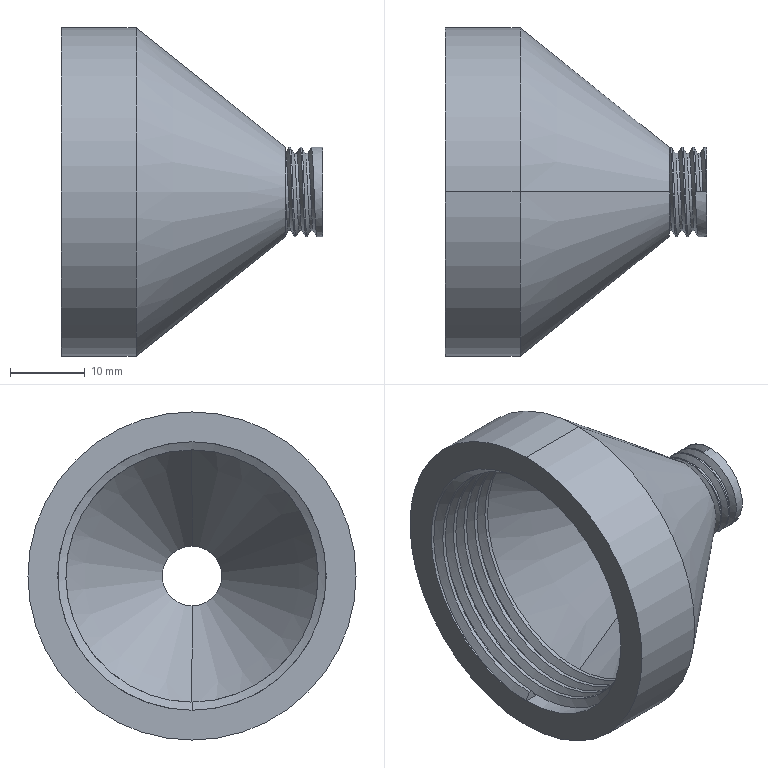Part | SolidWorks | features SweepThread 2, ICE 1, Revolution 1 | 1 solid | 39 faces | box 35 x 44 x 44 mm | volume 10879 mm3 | cylinder 22 | spline 7 | plane 6 | cone 4 | commonest cylinder face diameters 36 x11 12 x7 8 x2 44 x2